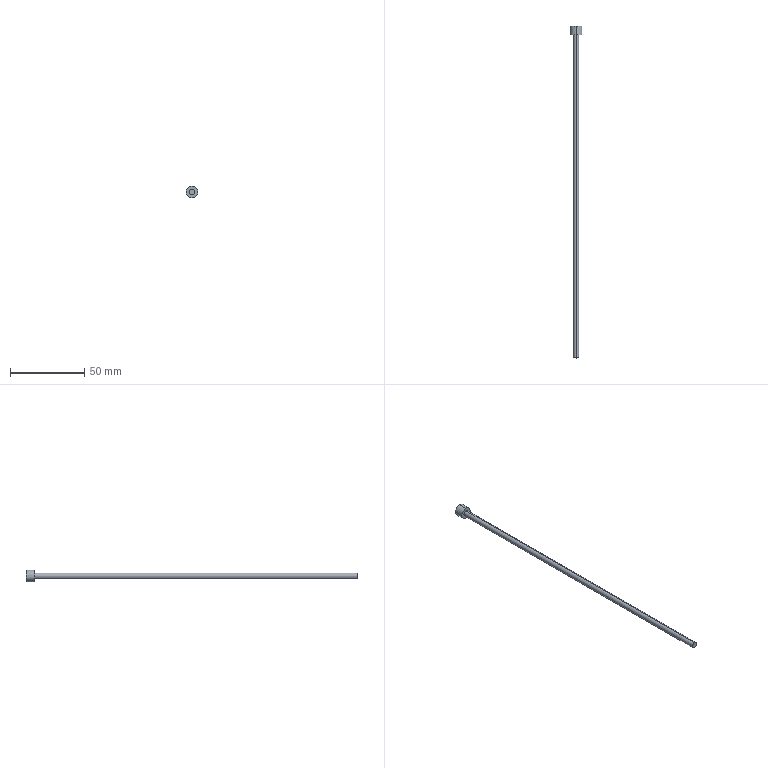Part | STEP file | 1 solid | 7 faces | box 8 x 223.165 x 8 mm | volume 3031 mm3 | cylinder 4 | plane 3 | commonest cylinder face diameters 4 x2 8 x2
STEP:
#1=CARTESIAN_POINT('',(0.,0.,0.));
#2=DIRECTION('',(0.,0.,1.));
#3=DIRECTION('',(1.,0.,0.));
#4=AXIS2_PLACEMENT_3D('',#1,#2,#3);
#5=CARTESIAN_POINT('',(-16.083,290.5,94.49));
#6=VERTEX_POINT('',#5);
#7=CARTESIAN_POINT('',(-16.083,290.5,102.49));
#8=VERTEX_POINT('',#7);
#9=CARTESIAN_POINT('',(-16.083,290.5,98.49));
#10=DIRECTION('',(0.,-1.,0.));
#11=DIRECTION('',(0.,0.,-1.));
#12=AXIS2_PLACEMENT_3D('',#9,#10,#11);
#13=CIRCLE('',#12,4.);
#14=CARTESIAN_POINT('',(-16.083,290.5,98.49));
#15=DIRECTION('',(0.,-1.,0.));
#16=DIRECTION('',(0.,0.,-1.));
#17=AXIS2_PLACEMENT_3D('',#14,#15,#16);
#18=CYLINDRICAL_SURFACE('',#17,4.);
#19=CARTESIAN_POINT('',(0.,0.));
#20=DIRECTION('',(1.,0.));
#21=VECTOR('',#20,1.);
#22=LINE('',#19,#21);
#23=(GEOMETRIC_REPRESENTATION_CONTEXT(2)PARAMETRIC_REPRESENTATION_CONTEXT()REPRESENTATION_CONTEXT('',''));
#24=DEFINITIONAL_REPRESENTATION('',(#22),#23);
#25=PCURVE('',#18,#24);
#26=CARTESIAN_POINT('',(-72.862,290.5,110.196));
#27=DIRECTION('',(0.,-1.,0.));
#28=DIRECTION('',(0.,0.,-1.));
#29=AXIS2_PLACEMENT_3D('',#26,#27,#28);
#30=PLANE('',#29);
#31=CARTESIAN_POINT('',(11.706,56.78));
#32=DIRECTION('',(1.,0.));
#33=AXIS2_PLACEMENT_2D('',#31,#32);
#34=CIRCLE('',#33,4.);
#35=(GEOMETRIC_REPRESENTATION_CONTEXT(2)PARAMETRIC_REPRESENTATION_CONTEXT()REPRESENTATION_CONTEXT('',''));
#36=DEFINITIONAL_REPRESENTATION('',(#34),#35);
#37=PCURVE('',#30,#36);
#38=SURFACE_CURVE('',#13,(#25,#37),.PCURVE_S1.);
#39=EDGE_CURVE('',#6,#8,#38,.T.);
#40=ORIENTED_EDGE('',*,*,#39,.T.);
#41=CARTESIAN_POINT('',(-16.083,284.5,102.49));
#42=VERTEX_POINT('',#41);
#43=CARTESIAN_POINT('',(-16.083,290.5,102.49));
#44=DIRECTION('',(0.,-1.,0.));
#45=VECTOR('',#44,1.);
#46=LINE('',#43,#45);
#47=CARTESIAN_POINT('',(3.142,0.));
#48=DIRECTION('',(0.,1.));
#49=VECTOR('',#48,1.);
#50=LINE('',#47,#49);
#51=(GEOMETRIC_REPRESENTATION_CONTEXT(2)PARAMETRIC_REPRESENTATION_CONTEXT()REPRESENTATION_CONTEXT('',''));
#52=DEFINITIONAL_REPRESENTATION('',(#50),#51);
#53=PCURVE('',#18,#52);
#54=CARTESIAN_POINT('',(-16.083,290.5,98.49));
#55=DIRECTION('',(0.,-1.,0.));
#56=DIRECTION('',(0.,0.,-1.));
#57=AXIS2_PLACEMENT_3D('',#54,#55,#56);
#58=CYLINDRICAL_SURFACE('',#57,4.);
#59=CARTESIAN_POINT('',(3.142,0.));
#60=DIRECTION('',(0.,1.));
#61=VECTOR('',#60,1.);
#62=LINE('',#59,#61);
#63=(GEOMETRIC_REPRESENTATION_CONTEXT(2)PARAMETRIC_REPRESENTATION_CONTEXT()REPRESENTATION_CONTEXT('',''));
#64=DEFINITIONAL_REPRESENTATION('',(#62),#63);
#65=PCURVE('',#58,#64);
#66=SURFACE_CURVE('',#46,(#53,#65),.PCURVE_S1.);
#67=EDGE_CURVE('',#8,#42,#66,.T.);
#68=ORIENTED_EDGE('',*,*,#67,.T.);
#69=CARTESIAN_POINT('',(-16.083,284.5,94.49));
#70=VERTEX_POINT('',#69);
#71=CARTESIAN_POINT('',(-16.083,284.5,98.49));
#72=DIRECTION('',(0.,1.,0.));
#73=DIRECTION('',(0.,0.,1.));
#74=AXIS2_PLACEMENT_3D('',#71,#72,#73);
#75=CIRCLE('',#74,4.);
#76=CARTESIAN_POINT('',(3.142,6.));
#77=DIRECTION('',(-1.,0.));
#78=VECTOR('',#77,1.);
#79=LINE('',#76,#78);
#80=(GEOMETRIC_REPRESENTATION_CONTEXT(2)PARAMETRIC_REPRESENTATION_CONTEXT()REPRESENTATION_CONTEXT('',''));
#81=DEFINITIONAL_REPRESENTATION('',(#79),#80);
#82=PCURVE('',#18,#81);
#83=CARTESIAN_POINT('',(-16.083,284.5,98.49));
#84=DIRECTION('',(0.,-1.,0.));
#85=DIRECTION('',(0.,0.,-1.));
#86=AXIS2_PLACEMENT_3D('',#83,#84,#85);
#87=PLANE('',#86);
#88=CARTESIAN_POINT('',(-4.,0.));
#89=CARTESIAN_POINT('',(-4.,6.928));
#90=CARTESIAN_POINT('',(2.,3.464));
#91=CARTESIAN_POINT('',(8.,0.));
#92=CARTESIAN_POINT('',(2.,-3.464));
#93=CARTESIAN_POINT('',(-4.,-6.928));
#94=CARTESIAN_POINT('',(-4.,0.));
#95=(BOUNDED_CURVE()B_SPLINE_CURVE(2,(#88,#89,#90,#91,#92,#93,#94),.UNSPECIFIED.,.T.,.F.)B_SPLINE_CURVE_WITH_KNOTS((1,2,2,2,2,1),(-2.094,0.,2.094,4.189,6.283,8.378),.UNSPECIFIED.)CURVE()GEOMETRIC_REPRESENTATION_ITEM()RATIONAL_B_SPLINE_CURVE((1.,0.5,1.,0.5,1.,0.5,1.))REPRESENTATION_ITEM(''));
#96=(GEOMETRIC_REPRESENTATION_CONTEXT(2)PARAMETRIC_REPRESENTATION_CONTEXT()REPRESENTATION_CONTEXT('',''));
#97=DEFINITIONAL_REPRESENTATION('',(#95),#96);
#98=PCURVE('',#87,#97);
#99=SURFACE_CURVE('',#75,(#82,#98),.PCURVE_S1.);
#100=EDGE_CURVE('',#42,#70,#99,.T.);
#101=ORIENTED_EDGE('',*,*,#100,.T.);
#102=CARTESIAN_POINT('',(-16.083,290.5,94.49));
#103=DIRECTION('',(0.,-1.,0.));
#104=VECTOR('',#103,1.);
#105=LINE('',#102,#104);
#106=CARTESIAN_POINT('',(0.,0.));
#107=DIRECTION('',(0.,1.));
#108=VECTOR('',#107,1.);
#109=LINE('',#106,#108);
#110=(GEOMETRIC_REPRESENTATION_CONTEXT(2)PARAMETRIC_REPRESENTATION_CONTEXT()REPRESENTATION_CONTEXT('',''));
#111=DEFINITIONAL_REPRESENTATION('',(#109),#110);
#112=PCURVE('',#18,#111);
#113=CARTESIAN_POINT('',(6.283,0.));
#114=DIRECTION('',(0.,1.));
#115=VECTOR('',#114,1.);
#116=LINE('',#113,#115);
#117=(GEOMETRIC_REPRESENTATION_CONTEXT(2)PARAMETRIC_REPRESENTATION_CONTEXT()REPRESENTATION_CONTEXT('',''));
#118=DEFINITIONAL_REPRESENTATION('',(#116),#117);
#119=PCURVE('',#58,#118);
#120=SURFACE_CURVE('',#105,(#112,#119),.PCURVE_S1.);
#121=EDGE_CURVE('',#6,#70,#120,.T.);
#122=ORIENTED_EDGE('',*,*,#121,.F.);
#123=EDGE_LOOP('',(#40,#68,#101,#122));
#124=FACE_BOUND('',#123,.T.);
#125=ADVANCED_FACE('',(#124),#18,.T.);
#126=CARTESIAN_POINT('',(-16.083,284.5,100.49));
#127=VERTEX_POINT('',#126);
#128=CARTESIAN_POINT('',(-16.083,284.5,96.49));
#129=VERTEX_POINT('',#128);
#130=CARTESIAN_POINT('',(-16.083,284.5,98.49));
#131=DIRECTION('',(0.,1.,0.));
#132=DIRECTION('',(0.,0.,-1.));
#133=AXIS2_PLACEMENT_3D('',#130,#131,#132);
#134=CIRCLE('',#133,2.);
#135=CARTESIAN_POINT('',(-16.083,220.5,98.49));
#136=DIRECTION('',(0.,-1.,0.));
#137=DIRECTION('',(0.,0.,-1.));
#138=AXIS2_PLACEMENT_3D('',#135,#136,#137);
#139=CYLINDRICAL_SURFACE('',#138,2.);
#140=CARTESIAN_POINT('',(6.283,-64.));
#141=DIRECTION('',(-1.,0.));
#142=VECTOR('',#141,1.);
#143=LINE('',#140,#142);
#144=(GEOMETRIC_REPRESENTATION_CONTEXT(2)PARAMETRIC_REPRESENTATION_CONTEXT()REPRESENTATION_CONTEXT('',''));
#145=DEFINITIONAL_REPRESENTATION('',(#143),#144);
#146=PCURVE('',#139,#145);
#147=CARTESIAN_POINT('',(2.,0.));
#148=CARTESIAN_POINT('',(2.,-3.464));
#149=CARTESIAN_POINT('',(-1.,-1.732));
#150=CARTESIAN_POINT('',(-4.,0.));
#151=CARTESIAN_POINT('',(-1.,1.732));
#152=CARTESIAN_POINT('',(2.,3.464));
#153=CARTESIAN_POINT('',(2.,0.));
#154=(BOUNDED_CURVE()B_SPLINE_CURVE(2,(#147,#148,#149,#150,#151,#152,#153),.UNSPECIFIED.,.T.,.F.)B_SPLINE_CURVE_WITH_KNOTS((1,2,2,2,2,1),(-2.094,0.,2.094,4.189,6.283,8.378),.UNSPECIFIED.)CURVE()GEOMETRIC_REPRESENTATION_ITEM()RATIONAL_B_SPLINE_CURVE((1.,0.5,1.,0.5,1.,0.5,1.))REPRESENTATION_ITEM(''));
#155=(GEOMETRIC_REPRESENTATION_CONTEXT(2)PARAMETRIC_REPRESENTATION_CONTEXT()REPRESENTATION_CONTEXT('',''));
#156=DEFINITIONAL_REPRESENTATION('',(#154),#155);
#157=PCURVE('',#87,#156);
#158=SURFACE_CURVE('',#134,(#146,#157),.PCURVE_S1.);
#159=EDGE_CURVE('',#127,#129,#158,.T.);
#160=ORIENTED_EDGE('',*,*,#159,.F.);
#161=CARTESIAN_POINT('',(-16.083,67.335,100.49));
#162=VERTEX_POINT('',#161);
#163=CARTESIAN_POINT('',(-16.083,220.5,100.49));
#164=DIRECTION('',(0.,-1.,0.));
#165=VECTOR('',#164,1.);
#166=LINE('',#163,#165);
#167=CARTESIAN_POINT('',(3.142,0.));
#168=DIRECTION('',(0.,1.));
#169=VECTOR('',#168,1.);
#170=LINE('',#167,#169);
#171=(GEOMETRIC_REPRESENTATION_CONTEXT(2)PARAMETRIC_REPRESENTATION_CONTEXT()REPRESENTATION_CONTEXT('',''));
#172=DEFINITIONAL_REPRESENTATION('',(#170),#171);
#173=PCURVE('',#139,#172);
#174=CARTESIAN_POINT('',(-16.083,220.5,98.49));
#175=DIRECTION('',(0.,-1.,0.));
#176=DIRECTION('',(0.,0.,-1.));
#177=AXIS2_PLACEMENT_3D('',#174,#175,#176);
#178=CYLINDRICAL_SURFACE('',#177,2.);
#179=CARTESIAN_POINT('',(3.142,0.));
#180=DIRECTION('',(0.,1.));
#181=VECTOR('',#180,1.);
#182=LINE('',#179,#181);
#183=(GEOMETRIC_REPRESENTATION_CONTEXT(2)PARAMETRIC_REPRESENTATION_CONTEXT()REPRESENTATION_CONTEXT('',''));
#184=DEFINITIONAL_REPRESENTATION('',(#182),#183);
#185=PCURVE('',#178,#184);
#186=SURFACE_CURVE('',#166,(#173,#185),.PCURVE_S1.);
#187=EDGE_CURVE('',#127,#162,#186,.T.);
#188=ORIENTED_EDGE('',*,*,#187,.T.);
#189=CARTESIAN_POINT('',(-16.083,67.335,96.49));
#190=VERTEX_POINT('',#189);
#191=CARTESIAN_POINT('',(-16.083,67.335,98.49));
#192=DIRECTION('',(0.,-1.,0.));
#193=DIRECTION('',(0.,0.,1.));
#194=AXIS2_PLACEMENT_3D('',#191,#192,#193);
#195=CIRCLE('',#194,2.);
#196=CARTESIAN_POINT('',(-3.142,153.165));
#197=DIRECTION('',(1.,0.));
#198=VECTOR('',#197,1.);
#199=LINE('',#196,#198);
#200=(GEOMETRIC_REPRESENTATION_CONTEXT(2)PARAMETRIC_REPRESENTATION_CONTEXT()REPRESENTATION_CONTEXT('',''));
#201=DEFINITIONAL_REPRESENTATION('',(#199),#200);
#202=PCURVE('',#139,#201);
#203=CARTESIAN_POINT('',(-16.08,67.335,98.49));
#204=DIRECTION('',(0.,1.,0.));
#205=DIRECTION('',(0.,0.,1.));
#206=AXIS2_PLACEMENT_3D('',#203,#204,#205);
#207=PLANE('',#206);
#208=CARTESIAN_POINT('',(2.,-0.002511));
#209=CARTESIAN_POINT('',(2.,-3.467));
#210=CARTESIAN_POINT('',(-1.,-1.735));
#211=CARTESIAN_POINT('',(-4.,-0.002511));
#212=CARTESIAN_POINT('',(-1.,1.73));
#213=CARTESIAN_POINT('',(2.,3.462));
#214=CARTESIAN_POINT('',(2.,-0.002511));
#215=(BOUNDED_CURVE()B_SPLINE_CURVE(2,(#208,#209,#210,#211,#212,#213,#214),.UNSPECIFIED.,.T.,.F.)B_SPLINE_CURVE_WITH_KNOTS((1,2,2,2,2,1),(-2.094,0.,2.094,4.189,6.283,8.378),.UNSPECIFIED.)CURVE()GEOMETRIC_REPRESENTATION_ITEM()RATIONAL_B_SPLINE_CURVE((1.,0.5,1.,0.5,1.,0.5,1.))REPRESENTATION_ITEM(''));
#216=(GEOMETRIC_REPRESENTATION_CONTEXT(2)PARAMETRIC_REPRESENTATION_CONTEXT()REPRESENTATION_CONTEXT('',''));
#217=DEFINITIONAL_REPRESENTATION('',(#215),#216);
#218=PCURVE('',#207,#217);
#219=SURFACE_CURVE('',#195,(#202,#218),.PCURVE_S1.);
#220=EDGE_CURVE('',#190,#162,#219,.T.);
#221=ORIENTED_EDGE('',*,*,#220,.F.);
#222=CARTESIAN_POINT('',(-16.083,220.5,96.49));
#223=DIRECTION('',(0.,-1.,0.));
#224=VECTOR('',#223,1.);
#225=LINE('',#222,#224);
#226=CARTESIAN_POINT('',(0.,0.));
#227=DIRECTION('',(0.,1.));
#228=VECTOR('',#227,1.);
#229=LINE('',#226,#228);
#230=(GEOMETRIC_REPRESENTATION_CONTEXT(2)PARAMETRIC_REPRESENTATION_CONTEXT()REPRESENTATION_CONTEXT('',''));
#231=DEFINITIONAL_REPRESENTATION('',(#229),#230);
#232=PCURVE('',#139,#231);
#233=CARTESIAN_POINT('',(6.283,0.));
#234=DIRECTION('',(0.,1.));
#235=VECTOR('',#234,1.);
#236=LINE('',#233,#235);
#237=(GEOMETRIC_REPRESENTATION_CONTEXT(2)PARAMETRIC_REPRESENTATION_CONTEXT()REPRESENTATION_CONTEXT('',''));
#238=DEFINITIONAL_REPRESENTATION('',(#236),#237);
#239=PCURVE('',#178,#238);
#240=SURFACE_CURVE('',#225,(#232,#239),.PCURVE_S1.);
#241=EDGE_CURVE('',#129,#190,#240,.T.);
#242=ORIENTED_EDGE('',*,*,#241,.F.);
#243=EDGE_LOOP('',(#160,#188,#221,#242));
#244=FACE_BOUND('',#243,.T.);
#245=ADVANCED_FACE('',(#244),#139,.T.);
#246=ORIENTED_EDGE('',*,*,#220,.T.);
#247=CARTESIAN_POINT('',(-16.083,67.335,98.49));
#248=DIRECTION('',(0.,-1.,0.));
#249=DIRECTION('',(0.,0.,1.));
#250=AXIS2_PLACEMENT_3D('',#247,#248,#249);
#251=CIRCLE('',#250,2.);
#252=CARTESIAN_POINT('',(2.,-0.002511));
#253=CARTESIAN_POINT('',(2.,-3.467));
#254=CARTESIAN_POINT('',(-1.,-1.735));
#255=CARTESIAN_POINT('',(-4.,-0.002511));
#256=CARTESIAN_POINT('',(-1.,1.73));
#257=CARTESIAN_POINT('',(2.,3.462));
#258=CARTESIAN_POINT('',(2.,-0.002511));
#259=(BOUNDED_CURVE()B_SPLINE_CURVE(2,(#252,#253,#254,#255,#256,#257,#258),.UNSPECIFIED.,.T.,.F.)B_SPLINE_CURVE_WITH_KNOTS((1,2,2,2,2,1),(-2.094,0.,2.094,4.189,6.283,8.378),.UNSPECIFIED.)CURVE()GEOMETRIC_REPRESENTATION_ITEM()RATIONAL_B_SPLINE_CURVE((1.,0.5,1.,0.5,1.,0.5,1.))REPRESENTATION_ITEM(''));
#260=(GEOMETRIC_REPRESENTATION_CONTEXT(2)PARAMETRIC_REPRESENTATION_CONTEXT()REPRESENTATION_CONTEXT('',''));
#261=DEFINITIONAL_REPRESENTATION('',(#259),#260);
#262=PCURVE('',#207,#261);
#263=CARTESIAN_POINT('',(3.142,153.165));
#264=DIRECTION('',(1.,0.));
#265=VECTOR('',#264,1.);
#266=LINE('',#263,#265);
#267=(GEOMETRIC_REPRESENTATION_CONTEXT(2)PARAMETRIC_REPRESENTATION_CONTEXT()REPRESENTATION_CONTEXT('',''));
#268=DEFINITIONAL_REPRESENTATION('',(#266),#267);
#269=PCURVE('',#178,#268);
#270=SURFACE_CURVE('',#251,(#262,#269),.PCURVE_S1.);
#271=EDGE_CURVE('',#162,#190,#270,.T.);
#272=ORIENTED_EDGE('',*,*,#271,.T.);
#273=EDGE_LOOP('',(#246,#272));
#274=FACE_BOUND('',#273,.T.);
#275=ADVANCED_FACE('',(#274),#207,.F.);
#276=ORIENTED_EDGE('',*,*,#187,.F.);
#277=CARTESIAN_POINT('',(-16.083,284.5,98.49));
#278=DIRECTION('',(0.,1.,0.));
#279=DIRECTION('',(0.,0.,-1.));
#280=AXIS2_PLACEMENT_3D('',#277,#278,#279);
#281=CIRCLE('',#280,2.);
#282=CARTESIAN_POINT('',(6.283,-64.));
#283=DIRECTION('',(-1.,0.));
#284=VECTOR('',#283,1.);
#285=LINE('',#282,#284);
#286=(GEOMETRIC_REPRESENTATION_CONTEXT(2)PARAMETRIC_REPRESENTATION_CONTEXT()REPRESENTATION_CONTEXT('',''));
#287=DEFINITIONAL_REPRESENTATION('',(#285),#286);
#288=PCURVE('',#178,#287);
#289=CARTESIAN_POINT('',(2.,0.));
#290=CARTESIAN_POINT('',(2.,-3.464));
#291=CARTESIAN_POINT('',(-1.,-1.732));
#292=CARTESIAN_POINT('',(-4.,0.));
#293=CARTESIAN_POINT('',(-1.,1.732));
#294=CARTESIAN_POINT('',(2.,3.464));
#295=CARTESIAN_POINT('',(2.,0.));
#296=(BOUNDED_CURVE()B_SPLINE_CURVE(2,(#289,#290,#291,#292,#293,#294,#295),.UNSPECIFIED.,.T.,.F.)B_SPLINE_CURVE_WITH_KNOTS((1,2,2,2,2,1),(-2.094,0.,2.094,4.189,6.283,8.378),.UNSPECIFIED.)CURVE()GEOMETRIC_REPRESENTATION_ITEM()RATIONAL_B_SPLINE_CURVE((1.,0.5,1.,0.5,1.,0.5,1.))REPRESENTATION_ITEM(''));
#297=(GEOMETRIC_REPRESENTATION_CONTEXT(2)PARAMETRIC_REPRESENTATION_CONTEXT()REPRESENTATION_CONTEXT('',''));
#298=DEFINITIONAL_REPRESENTATION('',(#296),#297);
#299=PCURVE('',#87,#298);
#300=SURFACE_CURVE('',#281,(#288,#299),.PCURVE_S1.);
#301=EDGE_CURVE('',#129,#127,#300,.T.);
#302=ORIENTED_EDGE('',*,*,#301,.F.);
#303=ORIENTED_EDGE('',*,*,#241,.T.);
#304=ORIENTED_EDGE('',*,*,#271,.F.);
#305=EDGE_LOOP('',(#276,#302,#303,#304));
#306=FACE_BOUND('',#305,.T.);
#307=ADVANCED_FACE('',(#306),#178,.T.);
#308=ORIENTED_EDGE('',*,*,#301,.T.);
#309=ORIENTED_EDGE('',*,*,#159,.T.);
#310=EDGE_LOOP('',(#308,#309));
#311=FACE_BOUND('',#310,.T.);
#312=CARTESIAN_POINT('',(-16.083,284.5,98.49));
#313=DIRECTION('',(0.,1.,0.));
#314=DIRECTION('',(0.,0.,1.));
#315=AXIS2_PLACEMENT_3D('',#312,#313,#314);
#316=CIRCLE('',#315,4.);
#317=CARTESIAN_POINT('',(-4.,0.));
#318=CARTESIAN_POINT('',(-4.,6.928));
#319=CARTESIAN_POINT('',(2.,3.464));
#320=CARTESIAN_POINT('',(8.,0.));
#321=CARTESIAN_POINT('',(2.,-3.464));
#322=CARTESIAN_POINT('',(-4.,-6.928));
#323=CARTESIAN_POINT('',(-4.,0.));
#324=(BOUNDED_CURVE()B_SPLINE_CURVE(2,(#317,#318,#319,#320,#321,#322,#323),.UNSPECIFIED.,.T.,.F.)B_SPLINE_CURVE_WITH_KNOTS((1,2,2,2,2,1),(-2.094,0.,2.094,4.189,6.283,8.378),.UNSPECIFIED.)CURVE()GEOMETRIC_REPRESENTATION_ITEM()RATIONAL_B_SPLINE_CURVE((1.,0.5,1.,0.5,1.,0.5,1.))REPRESENTATION_ITEM(''));
#325=(GEOMETRIC_REPRESENTATION_CONTEXT(2)PARAMETRIC_REPRESENTATION_CONTEXT()REPRESENTATION_CONTEXT('',''));
#326=DEFINITIONAL_REPRESENTATION('',(#324),#325);
#327=PCURVE('',#87,#326);
#328=CARTESIAN_POINT('',(9.425,6.));
#329=DIRECTION('',(-1.,0.));
#330=VECTOR('',#329,1.);
#331=LINE('',#328,#330);
#332=(GEOMETRIC_REPRESENTATION_CONTEXT(2)PARAMETRIC_REPRESENTATION_CONTEXT()REPRESENTATION_CONTEXT('',''));
#333=DEFINITIONAL_REPRESENTATION('',(#331),#332);
#334=PCURVE('',#58,#333);
#335=SURFACE_CURVE('',#316,(#327,#334),.PCURVE_S1.);
#336=EDGE_CURVE('',#70,#42,#335,.T.);
#337=ORIENTED_EDGE('',*,*,#336,.F.);
#338=ORIENTED_EDGE('',*,*,#100,.F.);
#339=EDGE_LOOP('',(#337,#338));
#340=FACE_BOUND('',#339,.T.);
#341=ADVANCED_FACE('',(#311,#340),#87,.T.);
#342=ORIENTED_EDGE('',*,*,#67,.F.);
#343=CARTESIAN_POINT('',(-16.083,290.5,98.49));
#344=DIRECTION('',(0.,-1.,0.));
#345=DIRECTION('',(0.,0.,-1.));
#346=AXIS2_PLACEMENT_3D('',#343,#344,#345);
#347=CIRCLE('',#346,4.);
#348=CARTESIAN_POINT('',(0.,0.));
#349=DIRECTION('',(1.,0.));
#350=VECTOR('',#349,1.);
#351=LINE('',#348,#350);
#352=(GEOMETRIC_REPRESENTATION_CONTEXT(2)PARAMETRIC_REPRESENTATION_CONTEXT()REPRESENTATION_CONTEXT('',''));
#353=DEFINITIONAL_REPRESENTATION('',(#351),#352);
#354=PCURVE('',#58,#353);
#355=CARTESIAN_POINT('',(11.706,56.78));
#356=DIRECTION('',(1.,0.));
#357=AXIS2_PLACEMENT_2D('',#355,#356);
#358=CIRCLE('',#357,4.);
#359=(GEOMETRIC_REPRESENTATION_CONTEXT(2)PARAMETRIC_REPRESENTATION_CONTEXT()REPRESENTATION_CONTEXT('',''));
#360=DEFINITIONAL_REPRESENTATION('',(#358),#359);
#361=PCURVE('',#30,#360);
#362=SURFACE_CURVE('',#347,(#354,#361),.PCURVE_S1.);
#363=EDGE_CURVE('',#8,#6,#362,.T.);
#364=ORIENTED_EDGE('',*,*,#363,.T.);
#365=ORIENTED_EDGE('',*,*,#121,.T.);
#366=ORIENTED_EDGE('',*,*,#336,.T.);
#367=EDGE_LOOP('',(#342,#364,#365,#366));
#368=FACE_BOUND('',#367,.T.);
#369=ADVANCED_FACE('',(#368),#58,.T.);
#370=ORIENTED_EDGE('',*,*,#39,.F.);
#371=ORIENTED_EDGE('',*,*,#363,.F.);
#372=EDGE_LOOP('',(#370,#371));
#373=FACE_BOUND('',#372,.T.);
#374=ADVANCED_FACE('',(#373),#30,.F.);
#375=CLOSED_SHELL('',(#125,#245,#275,#307,#341,#369,#374));
#376=MANIFOLD_SOLID_BREP('',#375);
#377=(LENGTH_UNIT()NAMED_UNIT(*)SI_UNIT(.MILLI.,.METRE.));
#378=UNCERTAINTY_MEASURE_WITH_UNIT(LENGTH_MEASURE(0.0000001),#377,'','');
#379=(NAMED_UNIT(*)PLANE_ANGLE_UNIT()SI_UNIT($,.RADIAN.));
#380=(NAMED_UNIT(*)SI_UNIT($,.STERADIAN.)SOLID_ANGLE_UNIT());
#381=(GEOMETRIC_REPRESENTATION_CONTEXT(3)GLOBAL_UNCERTAINTY_ASSIGNED_CONTEXT((#378))GLOBAL_UNIT_ASSIGNED_CONTEXT((#377,#379,#380))REPRESENTATION_CONTEXT('',''));
#382=ADVANCED_BREP_SHAPE_REPRESENTATION('',(#4,#376),#381);